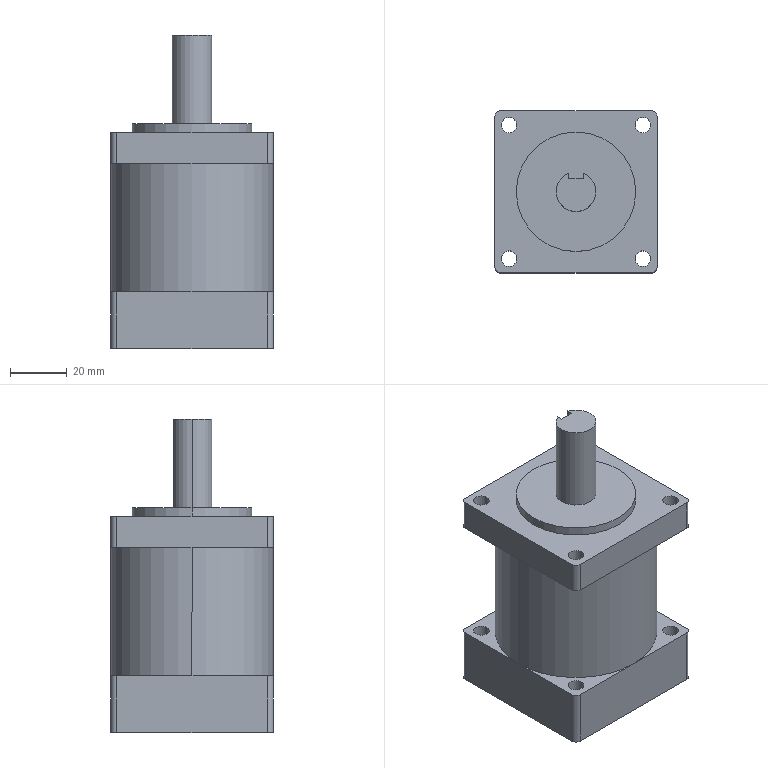Part | SolidWorks | features BaseBody 1 | 1 solid | 60 faces | box 57 x 57 x 110 mm | volume 214334 mm3 | cylinder 35 | plane 25 | commonest cylinder face diameters 5.5 x16 4 x8 14 x3 8 x2 38 x2 42 x2